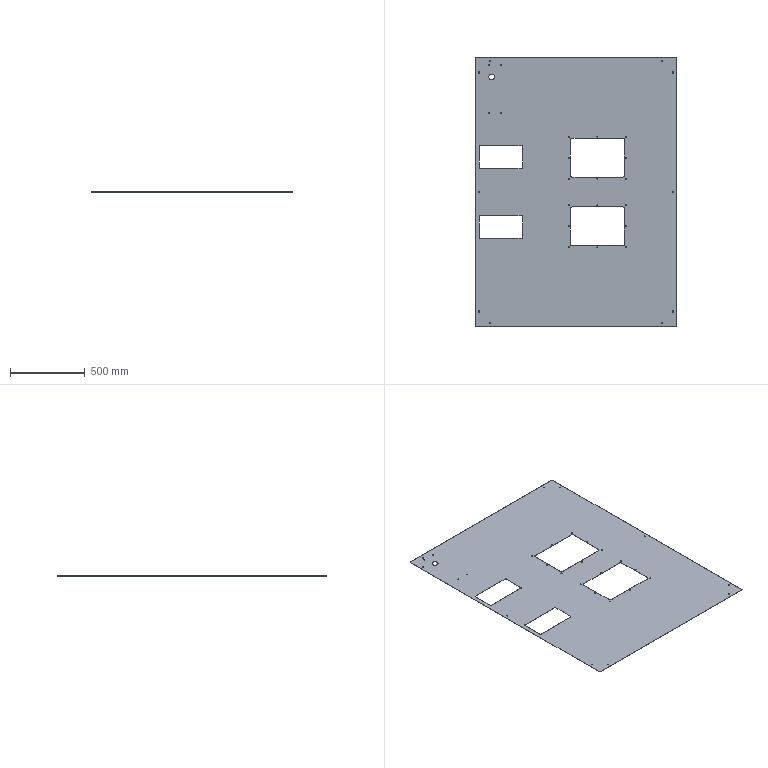Part | SolidWorks | features BaseBody 1 | 1 solid | 104 faces | box 1346 x 1796 x 1.5 mm | volume 3211505 mm3 | cylinder 82 | plane 22 | commonest cylinder face diameters 7 x60 10 x8 11.664 x4 20 x4 21.439 x4 40 x2